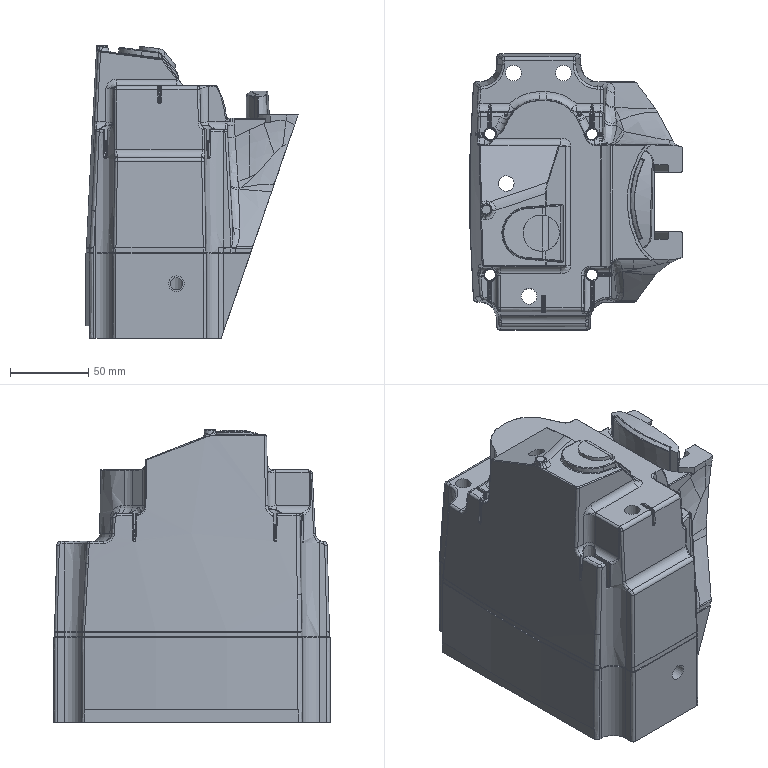Part | STEP file | solid 108 | 1 solid | 917 faces | box 136.142 x 176.757 x 187.43 mm | volume 2148805 mm3 | spline 404 | cylinder 241 | plane 156 | torus 41 | cone 35 | sphere 24 | other 16 | commonest cylinder face diameters 1.005 x69 0.502 x37 3.216 x15 5.226 x10 9.849 x10 10 x10